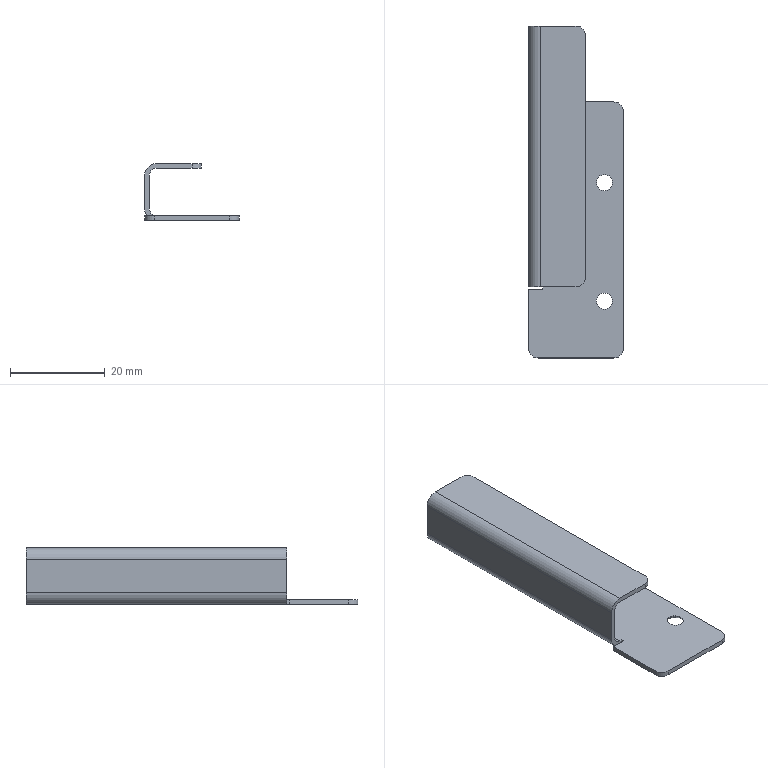Part | SolidWorks | features BaseBody 1 | 1 solid | 34 faces | box 20 x 70 x 12 mm | volume 2355 mm3 | plane 16 | cylinder 14 | cone 4 | commonest cylinder face diameters 4 x6 3.4 x4 3 x2 5 x2
STEP:
#1=CARTESIAN_POINT('',(-5.7,37.,1.));
#2=VERTEX_POINT('',#1);
#3=CARTESIAN_POINT('',(-2.3,37.,1.));
#4=VERTEX_POINT('',#3);
#5=CARTESIAN_POINT('',(-4.,37.,1.));
#6=DIRECTION('',(0.,0.,1.));
#7=DIRECTION('',(-1.,0.,0.));
#8=AXIS2_PLACEMENT_3D('',#5,#6,#7);
#9=CIRCLE('',#8,1.7);
#10=EDGE_CURVE('',#2,#4,#9,.T.);
#11=ORIENTED_EDGE('',*,*,#10,.T.);
#12=CARTESIAN_POINT('',(-2.3,37.,0.8));
#13=VERTEX_POINT('',#12);
#14=CARTESIAN_POINT('',(-2.3,37.,0.));
#15=DIRECTION('',(0.,0.,-1.));
#16=VECTOR('',#15,1000.);
#17=LINE('',#14,#16);
#18=EDGE_CURVE('',#4,#13,#17,.T.);
#19=ORIENTED_EDGE('',*,*,#18,.T.);
#20=CARTESIAN_POINT('',(-5.7,37.,0.8));
#21=VERTEX_POINT('',#20);
#22=CARTESIAN_POINT('',(-4.,37.,0.8));
#23=DIRECTION('',(0.,0.,1.));
#24=DIRECTION('',(-1.,0.,0.));
#25=AXIS2_PLACEMENT_3D('',#22,#23,#24);
#26=CIRCLE('',#25,1.7);
#27=EDGE_CURVE('',#21,#13,#26,.T.);
#28=ORIENTED_EDGE('',*,*,#27,.F.);
#29=CARTESIAN_POINT('',(-5.7,37.,0.));
#30=DIRECTION('',(0.,0.,-1.));
#31=VECTOR('',#30,1000.);
#32=LINE('',#29,#31);
#33=EDGE_CURVE('',#2,#21,#32,.T.);
#34=ORIENTED_EDGE('',*,*,#33,.F.);
#35=EDGE_LOOP('',(#11,#19,#28,#34));
#36=FACE_OUTER_BOUND('',#35,.T.);
#37=CARTESIAN_POINT('',(-4.,37.,0.));
#38=DIRECTION('',(0.,0.,-1.));
#39=DIRECTION('',(-1.,0.,0.));
#40=AXIS2_PLACEMENT_3D('',#37,#38,#39);
#41=CYLINDRICAL_SURFACE('',#40,1.7);
#42=ADVANCED_FACE('',(#36),#41,.F.);
#43=CARTESIAN_POINT('',(-5.7,12.,1.));
#44=VERTEX_POINT('',#43);
#45=CARTESIAN_POINT('',(-2.3,12.,1.));
#46=VERTEX_POINT('',#45);
#47=CARTESIAN_POINT('',(-4.,12.,1.));
#48=DIRECTION('',(0.,0.,1.));
#49=DIRECTION('',(-1.,0.,0.));
#50=AXIS2_PLACEMENT_3D('',#47,#48,#49);
#51=CIRCLE('',#50,1.7);
#52=EDGE_CURVE('',#44,#46,#51,.T.);
#53=ORIENTED_EDGE('',*,*,#52,.T.);
#54=CARTESIAN_POINT('',(-2.3,12.,0.8));
#55=VERTEX_POINT('',#54);
#56=CARTESIAN_POINT('',(-2.3,12.,0.));
#57=DIRECTION('',(0.,0.,-1.));
#58=VECTOR('',#57,1000.);
#59=LINE('',#56,#58);
#60=EDGE_CURVE('',#46,#55,#59,.T.);
#61=ORIENTED_EDGE('',*,*,#60,.T.);
#62=CARTESIAN_POINT('',(-5.7,12.,0.8));
#63=VERTEX_POINT('',#62);
#64=CARTESIAN_POINT('',(-4.,12.,0.8));
#65=DIRECTION('',(0.,0.,1.));
#66=DIRECTION('',(-1.,0.,0.));
#67=AXIS2_PLACEMENT_3D('',#64,#65,#66);
#68=CIRCLE('',#67,1.7);
#69=EDGE_CURVE('',#63,#55,#68,.T.);
#70=ORIENTED_EDGE('',*,*,#69,.F.);
#71=CARTESIAN_POINT('',(-5.7,12.,0.));
#72=DIRECTION('',(0.,0.,-1.));
#73=VECTOR('',#72,1000.);
#74=LINE('',#71,#73);
#75=EDGE_CURVE('',#44,#63,#74,.T.);
#76=ORIENTED_EDGE('',*,*,#75,.F.);
#77=EDGE_LOOP('',(#53,#61,#70,#76));
#78=FACE_OUTER_BOUND('',#77,.T.);
#79=CARTESIAN_POINT('',(-4.,12.,0.));
#80=DIRECTION('',(0.,0.,-1.));
#81=DIRECTION('',(-1.,0.,0.));
#82=AXIS2_PLACEMENT_3D('',#79,#80,#81);
#83=CYLINDRICAL_SURFACE('',#82,1.7);
#84=ADVANCED_FACE('',(#78),#83,.F.);
#85=ORIENTED_EDGE('',*,*,#27,.T.);
#86=CARTESIAN_POINT('',(-1.5,37.,0.));
#87=VERTEX_POINT('',#86);
#88=CARTESIAN_POINT('',(-1.5,37.,0.));
#89=DIRECTION('',(0.7071,0.,-0.7071));
#90=VECTOR('',#89,1000.);
#91=LINE('',#88,#90);
#92=EDGE_CURVE('',#13,#87,#91,.T.);
#93=ORIENTED_EDGE('',*,*,#92,.T.);
#94=CARTESIAN_POINT('',(-6.5,37.,0.));
#95=VERTEX_POINT('',#94);
#96=CARTESIAN_POINT('',(-4.,37.,0.));
#97=DIRECTION('',(0.,0.,1.));
#98=DIRECTION('',(-1.,0.,0.));
#99=AXIS2_PLACEMENT_3D('',#96,#97,#98);
#100=CIRCLE('',#99,2.5);
#101=EDGE_CURVE('',#95,#87,#100,.T.);
#102=ORIENTED_EDGE('',*,*,#101,.F.);
#103=CARTESIAN_POINT('',(-6.5,37.,0.));
#104=DIRECTION('',(-0.7071,0.,-0.7071));
#105=VECTOR('',#104,1000.);
#106=LINE('',#103,#105);
#107=EDGE_CURVE('',#21,#95,#106,.T.);
#108=ORIENTED_EDGE('',*,*,#107,.F.);
#109=EDGE_LOOP('',(#85,#93,#102,#108));
#110=FACE_OUTER_BOUND('',#109,.T.);
#111=CARTESIAN_POINT('',(-4.,37.,0.));
#112=DIRECTION('',(0.,0.,-1.));
#113=DIRECTION('',(-1.,0.,0.));
#114=AXIS2_PLACEMENT_3D('',#111,#112,#113);
#115=CONICAL_SURFACE('',#114,2.5,0.7854);
#116=ADVANCED_FACE('',(#110),#115,.F.);
#117=ORIENTED_EDGE('',*,*,#69,.T.);
#118=CARTESIAN_POINT('',(-1.5,12.,0.));
#119=VERTEX_POINT('',#118);
#120=CARTESIAN_POINT('',(-1.5,12.,0.));
#121=DIRECTION('',(0.7071,0.,-0.7071));
#122=VECTOR('',#121,1000.);
#123=LINE('',#120,#122);
#124=EDGE_CURVE('',#55,#119,#123,.T.);
#125=ORIENTED_EDGE('',*,*,#124,.T.);
#126=CARTESIAN_POINT('',(-6.5,12.,0.));
#127=VERTEX_POINT('',#126);
#128=CARTESIAN_POINT('',(-4.,12.,0.));
#129=DIRECTION('',(0.,0.,1.));
#130=DIRECTION('',(-1.,0.,0.));
#131=AXIS2_PLACEMENT_3D('',#128,#129,#130);
#132=CIRCLE('',#131,2.5);
#133=EDGE_CURVE('',#127,#119,#132,.T.);
#134=ORIENTED_EDGE('',*,*,#133,.F.);
#135=CARTESIAN_POINT('',(-6.5,12.,0.));
#136=DIRECTION('',(-0.7071,0.,-0.7071));
#137=VECTOR('',#136,1000.);
#138=LINE('',#135,#137);
#139=EDGE_CURVE('',#63,#127,#138,.T.);
#140=ORIENTED_EDGE('',*,*,#139,.F.);
#141=EDGE_LOOP('',(#117,#125,#134,#140));
#142=FACE_OUTER_BOUND('',#141,.T.);
#143=CARTESIAN_POINT('',(-4.,12.,0.));
#144=DIRECTION('',(0.,0.,-1.));
#145=DIRECTION('',(-1.,0.,0.));
#146=AXIS2_PLACEMENT_3D('',#143,#144,#145);
#147=CONICAL_SURFACE('',#146,2.5,0.7854);
#148=ADVANCED_FACE('',(#142),#147,.F.);
#149=ORIENTED_EDGE('',*,*,#10,.F.);
#150=CARTESIAN_POINT('',(-4.,37.,1.));
#151=DIRECTION('',(0.,0.,1.));
#152=DIRECTION('',(-1.,0.,0.));
#153=AXIS2_PLACEMENT_3D('',#150,#151,#152);
#154=CIRCLE('',#153,1.7);
#155=EDGE_CURVE('',#4,#2,#154,.T.);
#156=ORIENTED_EDGE('',*,*,#155,.F.);
#157=EDGE_LOOP('',(#149,#156));
#158=FACE_BOUND('',#157,.T.);
#159=ORIENTED_EDGE('',*,*,#52,.F.);
#160=CARTESIAN_POINT('',(-4.,12.,1.));
#161=DIRECTION('',(0.,0.,1.));
#162=DIRECTION('',(-1.,0.,0.));
#163=AXIS2_PLACEMENT_3D('',#160,#161,#162);
#164=CIRCLE('',#163,1.7);
#165=EDGE_CURVE('',#46,#44,#164,.T.);
#166=ORIENTED_EDGE('',*,*,#165,.F.);
#167=EDGE_LOOP('',(#159,#166));
#168=FACE_BOUND('',#167,.T.);
#169=CARTESIAN_POINT('',(0.,52.,1.));
#170=VERTEX_POINT('',#169);
#171=CARTESIAN_POINT('',(0.,2.,1.));
#172=VERTEX_POINT('',#171);
#173=CARTESIAN_POINT('',(0.,70.,1.));
#174=DIRECTION('',(0.,-1.,0.));
#175=VECTOR('',#174,1000.);
#176=LINE('',#173,#175);
#177=EDGE_CURVE('',#170,#172,#176,.T.);
#178=ORIENTED_EDGE('',*,*,#177,.F.);
#179=CARTESIAN_POINT('',(-2.,54.,1.));
#180=VERTEX_POINT('',#179);
#181=CARTESIAN_POINT('',(-2.,52.,1.));
#182=DIRECTION('',(0.,0.,-1.));
#183=DIRECTION('',(-1.,0.,0.));
#184=AXIS2_PLACEMENT_3D('',#181,#182,#183);
#185=CIRCLE('',#184,2.);
#186=EDGE_CURVE('',#180,#170,#185,.T.);
#187=ORIENTED_EDGE('',*,*,#186,.F.);
#188=CARTESIAN_POINT('',(-8.,54.,1.));
#189=VERTEX_POINT('',#188);
#190=CARTESIAN_POINT('',(0.,54.,1.));
#191=DIRECTION('',(1.,0.,0.));
#192=VECTOR('',#191,1000.);
#193=LINE('',#190,#192);
#194=EDGE_CURVE('',#189,#180,#193,.T.);
#195=ORIENTED_EDGE('',*,*,#194,.F.);
#196=CARTESIAN_POINT('',(-8.,68.,1.));
#197=VERTEX_POINT('',#196);
#198=CARTESIAN_POINT('',(-8.,70.,1.));
#199=DIRECTION('',(0.,-1.,0.));
#200=VECTOR('',#199,1000.);
#201=LINE('',#198,#200);
#202=EDGE_CURVE('',#197,#189,#201,.T.);
#203=ORIENTED_EDGE('',*,*,#202,.F.);
#204=CARTESIAN_POINT('',(-10.,70.,1.));
#205=VERTEX_POINT('',#204);
#206=CARTESIAN_POINT('',(-10.,68.,1.));
#207=DIRECTION('',(0.,0.,-1.));
#208=DIRECTION('',(-1.,0.,0.));
#209=AXIS2_PLACEMENT_3D('',#206,#207,#208);
#210=CIRCLE('',#209,2.);
#211=EDGE_CURVE('',#205,#197,#210,.T.);
#212=ORIENTED_EDGE('',*,*,#211,.F.);
#213=CARTESIAN_POINT('',(-17.5,70.,1.));
#214=VERTEX_POINT('',#213);
#215=CARTESIAN_POINT('',(0.,70.,1.));
#216=DIRECTION('',(1.,0.,0.));
#217=VECTOR('',#216,1000.);
#218=LINE('',#215,#217);
#219=EDGE_CURVE('',#214,#205,#218,.T.);
#220=ORIENTED_EDGE('',*,*,#219,.F.);
#221=CARTESIAN_POINT('',(-17.5,15.,1.));
#222=VERTEX_POINT('',#221);
#223=CARTESIAN_POINT('',(-17.5,70.,1.));
#224=DIRECTION('',(0.,1.,0.));
#225=VECTOR('',#224,1000.);
#226=LINE('',#223,#225);
#227=EDGE_CURVE('',#222,#214,#226,.T.);
#228=ORIENTED_EDGE('',*,*,#227,.F.);
#229=CARTESIAN_POINT('',(-17.,15.,1.));
#230=VERTEX_POINT('',#229);
#231=CARTESIAN_POINT('',(-8.,15.,1.));
#232=DIRECTION('',(1.,0.,0.));
#233=VECTOR('',#232,1000.);
#234=LINE('',#231,#233);
#235=EDGE_CURVE('',#222,#230,#234,.T.);
#236=ORIENTED_EDGE('',*,*,#235,.T.);
#237=CARTESIAN_POINT('',(-17.,14.5,1.));
#238=VERTEX_POINT('',#237);
#239=CARTESIAN_POINT('',(-17.,70.,1.));
#240=DIRECTION('',(0.,1.,0.));
#241=VECTOR('',#240,1000.);
#242=LINE('',#239,#241);
#243=EDGE_CURVE('',#238,#230,#242,.T.);
#244=ORIENTED_EDGE('',*,*,#243,.F.);
#245=CARTESIAN_POINT('',(-20.,14.5,1.));
#246=VERTEX_POINT('',#245);
#247=CARTESIAN_POINT('',(0.,14.5,1.));
#248=DIRECTION('',(1.,0.,0.));
#249=VECTOR('',#248,1000.);
#250=LINE('',#247,#249);
#251=EDGE_CURVE('',#246,#238,#250,.T.);
#252=ORIENTED_EDGE('',*,*,#251,.F.);
#253=CARTESIAN_POINT('',(-20.,2.,1.));
#254=VERTEX_POINT('',#253);
#255=CARTESIAN_POINT('',(-20.,70.,1.));
#256=DIRECTION('',(0.,1.,0.));
#257=VECTOR('',#256,1000.);
#258=LINE('',#255,#257);
#259=EDGE_CURVE('',#254,#246,#258,.T.);
#260=ORIENTED_EDGE('',*,*,#259,.F.);
#261=CARTESIAN_POINT('',(-18.,0.,1.));
#262=VERTEX_POINT('',#261);
#263=CARTESIAN_POINT('',(-18.,2.,1.));
#264=DIRECTION('',(0.,0.,-1.));
#265=DIRECTION('',(-1.,0.,0.));
#266=AXIS2_PLACEMENT_3D('',#263,#264,#265);
#267=CIRCLE('',#266,2.);
#268=EDGE_CURVE('',#262,#254,#267,.T.);
#269=ORIENTED_EDGE('',*,*,#268,.F.);
#270=CARTESIAN_POINT('',(-2.,0.,1.));
#271=VERTEX_POINT('',#270);
#272=CARTESIAN_POINT('',(0.,0.,1.));
#273=DIRECTION('',(-1.,0.,0.));
#274=VECTOR('',#273,1000.);
#275=LINE('',#272,#274);
#276=EDGE_CURVE('',#271,#262,#275,.T.);
#277=ORIENTED_EDGE('',*,*,#276,.F.);
#278=CARTESIAN_POINT('',(-2.,2.,1.));
#279=DIRECTION('',(0.,0.,-1.));
#280=DIRECTION('',(1.,0.,0.));
#281=AXIS2_PLACEMENT_3D('',#278,#279,#280);
#282=CIRCLE('',#281,2.);
#283=EDGE_CURVE('',#172,#271,#282,.T.);
#284=ORIENTED_EDGE('',*,*,#283,.F.);
#285=EDGE_LOOP('',(#178,#187,#195,#203,#212,#220,#228,#236,#244,#252,#260,#269,#277,#284));
#286=FACE_OUTER_BOUND('',#285,.T.);
#287=CARTESIAN_POINT('',(0.,70.,1.));
#288=DIRECTION('',(0.,0.,-1.));
#289=DIRECTION('',(-1.,0.,0.));
#290=AXIS2_PLACEMENT_3D('',#287,#288,#289);
#291=PLANE('',#290);
#292=ADVANCED_FACE('',(#158,#168,#286),#291,.F.);
#293=ORIENTED_EDGE('',*,*,#18,.F.);
#294=ORIENTED_EDGE('',*,*,#155,.T.);
#295=ORIENTED_EDGE('',*,*,#33,.T.);
#296=CARTESIAN_POINT('',(-4.,37.,0.8));
#297=DIRECTION('',(0.,0.,1.));
#298=DIRECTION('',(-1.,0.,0.));
#299=AXIS2_PLACEMENT_3D('',#296,#297,#298);
#300=CIRCLE('',#299,1.7);
#301=EDGE_CURVE('',#13,#21,#300,.T.);
#302=ORIENTED_EDGE('',*,*,#301,.F.);
#303=EDGE_LOOP('',(#293,#294,#295,#302));
#304=FACE_OUTER_BOUND('',#303,.T.);
#305=CARTESIAN_POINT('',(-4.,37.,0.));
#306=DIRECTION('',(0.,0.,-1.));
#307=DIRECTION('',(-1.,0.,0.));
#308=AXIS2_PLACEMENT_3D('',#305,#306,#307);
#309=CYLINDRICAL_SURFACE('',#308,1.7);
#310=ADVANCED_FACE('',(#304),#309,.F.);
#311=ORIENTED_EDGE('',*,*,#60,.F.);
#312=ORIENTED_EDGE('',*,*,#165,.T.);
#313=ORIENTED_EDGE('',*,*,#75,.T.);
#314=CARTESIAN_POINT('',(-4.,12.,0.8));
#315=DIRECTION('',(0.,0.,1.));
#316=DIRECTION('',(-1.,0.,0.));
#317=AXIS2_PLACEMENT_3D('',#314,#315,#316);
#318=CIRCLE('',#317,1.7);
#319=EDGE_CURVE('',#55,#63,#318,.T.);
#320=ORIENTED_EDGE('',*,*,#319,.F.);
#321=EDGE_LOOP('',(#311,#312,#313,#320));
#322=FACE_OUTER_BOUND('',#321,.T.);
#323=CARTESIAN_POINT('',(-4.,12.,0.));
#324=DIRECTION('',(0.,0.,-1.));
#325=DIRECTION('',(-1.,0.,0.));
#326=AXIS2_PLACEMENT_3D('',#323,#324,#325);
#327=CYLINDRICAL_SURFACE('',#326,1.7);
#328=ADVANCED_FACE('',(#322),#327,.F.);
#329=ORIENTED_EDGE('',*,*,#283,.T.);
#330=CARTESIAN_POINT('',(-2.,0.,0.));
#331=VERTEX_POINT('',#330);
#332=CARTESIAN_POINT('',(-2.,0.,0.));
#333=DIRECTION('',(0.,0.,-1.));
#334=VECTOR('',#333,1000.);
#335=LINE('',#332,#334);
#336=EDGE_CURVE('',#271,#331,#335,.T.);
#337=ORIENTED_EDGE('',*,*,#336,.T.);
#338=CARTESIAN_POINT('',(0.,2.,0.));
#339=VERTEX_POINT('',#338);
#340=CARTESIAN_POINT('',(-2.,2.,0.));
#341=DIRECTION('',(0.,0.,1.));
#342=DIRECTION('',(1.,0.,0.));
#343=AXIS2_PLACEMENT_3D('',#340,#341,#342);
#344=CIRCLE('',#343,2.);
#345=EDGE_CURVE('',#331,#339,#344,.T.);
#346=ORIENTED_EDGE('',*,*,#345,.T.);
#347=CARTESIAN_POINT('',(0.,2.,0.));
#348=DIRECTION('',(0.,0.,1.));
#349=VECTOR('',#348,1000.);
#350=LINE('',#347,#349);
#351=EDGE_CURVE('',#339,#172,#350,.T.);
#352=ORIENTED_EDGE('',*,*,#351,.T.);
#353=EDGE_LOOP('',(#329,#337,#346,#352));
#354=FACE_OUTER_BOUND('',#353,.T.);
#355=CARTESIAN_POINT('',(-2.,2.,0.));
#356=DIRECTION('',(0.,0.,1.));
#357=DIRECTION('',(1.,0.,0.));
#358=AXIS2_PLACEMENT_3D('',#355,#356,#357);
#359=CYLINDRICAL_SURFACE('',#358,2.);
#360=ADVANCED_FACE('',(#354),#359,.T.);
#361=ORIENTED_EDGE('',*,*,#177,.T.);
#362=ORIENTED_EDGE('',*,*,#351,.F.);
#363=CARTESIAN_POINT('',(0.,52.,0.));
#364=VERTEX_POINT('',#363);
#365=CARTESIAN_POINT('',(0.,70.,0.));
#366=DIRECTION('',(0.,-1.,0.));
#367=VECTOR('',#366,1000.);
#368=LINE('',#365,#367);
#369=EDGE_CURVE('',#364,#339,#368,.T.);
#370=ORIENTED_EDGE('',*,*,#369,.F.);
#371=CARTESIAN_POINT('',(0.,52.,0.));
#372=DIRECTION('',(0.,0.,-1.));
#373=VECTOR('',#372,1000.);
#374=LINE('',#371,#373);
#375=EDGE_CURVE('',#170,#364,#374,.T.);
#376=ORIENTED_EDGE('',*,*,#375,.F.);
#377=EDGE_LOOP('',(#361,#362,#370,#376));
#378=FACE_OUTER_BOUND('',#377,.T.);
#379=CARTESIAN_POINT('',(0.,70.,0.));
#380=DIRECTION('',(-1.,0.,0.));
#381=DIRECTION('',(0.,0.,1.));
#382=AXIS2_PLACEMENT_3D('',#379,#380,#381);
#383=PLANE('',#382);
#384=ADVANCED_FACE('',(#378),#383,.F.);
#385=ORIENTED_EDGE('',*,*,#186,.T.);
#386=ORIENTED_EDGE('',*,*,#375,.T.);
#387=CARTESIAN_POINT('',(-2.,54.,0.));
#388=VERTEX_POINT('',#387);
#389=CARTESIAN_POINT('',(-2.,52.,0.));
#390=DIRECTION('',(0.,0.,1.));
#391=DIRECTION('',(-1.,0.,0.));
#392=AXIS2_PLACEMENT_3D('',#389,#390,#391);
#393=CIRCLE('',#392,2.);
#394=EDGE_CURVE('',#364,#388,#393,.T.);
#395=ORIENTED_EDGE('',*,*,#394,.T.);
#396=CARTESIAN_POINT('',(-2.,54.,2.));
#397=DIRECTION('',(0.,0.,1.));
#398=VECTOR('',#397,1000.);
#399=LINE('',#396,#398);
#400=EDGE_CURVE('',#388,#180,#399,.T.);
#401=ORIENTED_EDGE('',*,*,#400,.T.);
#402=EDGE_LOOP('',(#385,#386,#395,#401));
#403=FACE_OUTER_BOUND('',#402,.T.);
#404=CARTESIAN_POINT('',(-2.,52.,2.));
#405=DIRECTION('',(0.,0.,-1.));
#406=DIRECTION('',(-1.,0.,0.));
#407=AXIS2_PLACEMENT_3D('',#404,#405,#406);
#408=CYLINDRICAL_SURFACE('',#407,2.);
#409=ADVANCED_FACE('',(#403),#408,.T.);
#410=ORIENTED_EDGE('',*,*,#194,.T.);
#411=ORIENTED_EDGE('',*,*,#400,.F.);
#412=CARTESIAN_POINT('',(-8.,54.,0.));
#413=VERTEX_POINT('',#412);
#414=CARTESIAN_POINT('',(0.,54.,0.));
#415=DIRECTION('',(1.,0.,0.));
#416=VECTOR('',#415,1000.);
#417=LINE('',#414,#416);
#418=EDGE_CURVE('',#413,#388,#417,.T.);
#419=ORIENTED_EDGE('',*,*,#418,.F.);
#420=CARTESIAN_POINT('',(-8.,54.,2.));
#421=DIRECTION('',(0.,0.,-1.));
#422=VECTOR('',#421,1000.);
#423=LINE('',#420,#422);
#424=EDGE_CURVE('',#189,#413,#423,.T.);
#425=ORIENTED_EDGE('',*,*,#424,.F.);
#426=EDGE_LOOP('',(#410,#411,#419,#425));
#427=FACE_OUTER_BOUND('',#426,.T.);
#428=CARTESIAN_POINT('',(0.,54.,2.));
#429=DIRECTION('',(0.,-1.,0.));
#430=DIRECTION('',(0.,0.,-1.));
#431=AXIS2_PLACEMENT_3D('',#428,#429,#430);
#432=PLANE('',#431);
#433=ADVANCED_FACE('',(#427),#432,.F.);
#434=CARTESIAN_POINT('',(-8.,68.,0.));
#435=VERTEX_POINT('',#434);
#436=CARTESIAN_POINT('',(-8.,70.,0.));
#437=DIRECTION('',(0.,-1.,0.));
#438=VECTOR('',#437,1000.);
#439=LINE('',#436,#438);
#440=EDGE_CURVE('',#435,#413,#439,.T.);
#441=ORIENTED_EDGE('',*,*,#440,.F.);
#442=CARTESIAN_POINT('',(-8.,68.,2.));
#443=DIRECTION('',(0.,0.,-1.));
#444=VECTOR('',#443,1000.);
#445=LINE('',#442,#444);
#446=EDGE_CURVE('',#197,#435,#445,.T.);
#447=ORIENTED_EDGE('',*,*,#446,.F.);
#448=ORIENTED_EDGE('',*,*,#202,.T.);
#449=ORIENTED_EDGE('',*,*,#424,.T.);
#450=EDGE_LOOP('',(#441,#447,#448,#449));
#451=FACE_OUTER_BOUND('',#450,.T.);
#452=CARTESIAN_POINT('',(-8.,70.,2.));
#453=DIRECTION('',(-1.,0.,0.));
#454=DIRECTION('',(0.,0.,1.));
#455=AXIS2_PLACEMENT_3D('',#452,#453,#454);
#456=PLANE('',#455);
#457=ADVANCED_FACE('',(#451),#456,.F.);
#458=ORIENTED_EDGE('',*,*,#211,.T.);
#459=ORIENTED_EDGE('',*,*,#446,.T.);
#460=CARTESIAN_POINT('',(-10.,70.,0.));
#461=VERTEX_POINT('',#460);
#462=CARTESIAN_POINT('',(-10.,68.,0.));
#463=DIRECTION('',(0.,0.,1.));
#464=DIRECTION('',(-1.,0.,0.));
#465=AXIS2_PLACEMENT_3D('',#462,#463,#464);
#466=CIRCLE('',#465,2.);
#467=EDGE_CURVE('',#435,#461,#466,.T.);
#468=ORIENTED_EDGE('',*,*,#467,.T.);
#469=CARTESIAN_POINT('',(-10.,70.,0.));
#470=DIRECTION('',(0.,0.,1.));
#471=VECTOR('',#470,1000.);
#472=LINE('',#469,#471);
#473=EDGE_CURVE('',#461,#205,#472,.T.);
#474=ORIENTED_EDGE('',*,*,#473,.T.);
#475=EDGE_LOOP('',(#458,#459,#468,#474));
#476=FACE_OUTER_BOUND('',#475,.T.);
#477=CARTESIAN_POINT('',(-10.,68.,0.));
#478=DIRECTION('',(0.,0.,-1.));
#479=DIRECTION('',(-1.,0.,0.));
#480=AXIS2_PLACEMENT_3D('',#477,#478,#479);
#481=CYLINDRICAL_SURFACE('',#480,2.);
#482=ADVANCED_FACE('',(#476),#481,.T.);
#483=CARTESIAN_POINT('',(-17.5,70.,11.));
#484=VERTEX_POINT('',#483);
#485=CARTESIAN_POINT('',(-10.,70.,11.));
#486=VERTEX_POINT('',#485);
#487=CARTESIAN_POINT('',(0.,70.,11.));
#488=DIRECTION('',(1.,0.,0.));
#489=VECTOR('',#488,1000.);
#490=LINE('',#487,#489);
#491=EDGE_CURVE('',#484,#486,#490,.T.);
#492=ORIENTED_EDGE('',*,*,#491,.F.);
#493=CARTESIAN_POINT('',(-19.,70.,9.5));
#494=VERTEX_POINT('',#493);
#495=CARTESIAN_POINT('',(-17.5,70.,9.5));
#496=DIRECTION('',(0.,1.,0.));
#497=DIRECTION('',(0.,0.,1.));
#498=AXIS2_PLACEMENT_3D('',#495,#496,#497);
#499=CIRCLE('',#498,1.5);
#500=EDGE_CURVE('',#494,#484,#499,.T.);
#501=ORIENTED_EDGE('',*,*,#500,.F.);
#502=CARTESIAN_POINT('',(-19.,70.,2.5));
#503=VERTEX_POINT('',#502);
#504=CARTESIAN_POINT('',(-19.,70.,0.));
#505=DIRECTION('',(0.,0.,1.));
#506=VECTOR('',#505,1000.);
#507=LINE('',#504,#506);
#508=EDGE_CURVE('',#503,#494,#507,.T.);
#509=ORIENTED_EDGE('',*,*,#508,.F.);
#510=CARTESIAN_POINT('',(-17.5,70.,2.5));
#511=DIRECTION('',(0.,1.,0.));
#512=DIRECTION('',(0.,0.,1.));
#513=AXIS2_PLACEMENT_3D('',#510,#511,#512);
#514=CIRCLE('',#513,1.5);
#515=EDGE_CURVE('',#214,#503,#514,.T.);
#516=ORIENTED_EDGE('',*,*,#515,.F.);
#517=ORIENTED_EDGE('',*,*,#219,.T.);
#518=ORIENTED_EDGE('',*,*,#473,.F.);
#519=CARTESIAN_POINT('',(-17.5,70.,0.));
#520=VERTEX_POINT('',#519);
#521=CARTESIAN_POINT('',(0.,70.,0.));
#522=DIRECTION('',(1.,0.,0.));
#523=VECTOR('',#522,1000.);
#524=LINE('',#521,#523);
#525=EDGE_CURVE('',#520,#461,#524,.T.);
#526=ORIENTED_EDGE('',*,*,#525,.F.);
#527=CARTESIAN_POINT('',(-20.,70.,2.5));
#528=VERTEX_POINT('',#527);
#529=CARTESIAN_POINT('',(-17.5,70.,2.5));
#530=DIRECTION('',(0.,-1.,0.));
#531=DIRECTION('',(0.,0.,-1.));
#532=AXIS2_PLACEMENT_3D('',#529,#530,#531);
#533=CIRCLE('',#532,2.5);
#534=EDGE_CURVE('',#528,#520,#533,.T.);
#535=ORIENTED_EDGE('',*,*,#534,.F.);
#536=CARTESIAN_POINT('',(-20.,70.,9.5));
#537=VERTEX_POINT('',#536);
#538=CARTESIAN_POINT('',(-20.,70.,0.));
#539=DIRECTION('',(0.,0.,-1.));
#540=VECTOR('',#539,1000.);
#541=LINE('',#538,#540);
#542=EDGE_CURVE('',#537,#528,#541,.T.);
#543=ORIENTED_EDGE('',*,*,#542,.F.);
#544=CARTESIAN_POINT('',(-17.5,70.,12.));
#545=VERTEX_POINT('',#544);
#546=CARTESIAN_POINT('',(-17.5,70.,9.5));
#547=DIRECTION('',(0.,-1.,0.));
#548=DIRECTION('',(0.,0.,-1.));
#549=AXIS2_PLACEMENT_3D('',#546,#547,#548);
#550=CIRCLE('',#549,2.5);
#551=EDGE_CURVE('',#545,#537,#550,.T.);
#552=ORIENTED_EDGE('',*,*,#551,.F.);
#553=CARTESIAN_POINT('',(-10.,70.,12.));
#554=VERTEX_POINT('',#553);
#555=CARTESIAN_POINT('',(0.,70.,12.));
#556=DIRECTION('',(-1.,0.,0.));
#557=VECTOR('',#556,1000.);
#558=LINE('',#555,#557);
#559=EDGE_CURVE('',#554,#545,#558,.T.);
#560=ORIENTED_EDGE('',*,*,#559,.F.);
#561=CARTESIAN_POINT('',(-10.,70.,0.));
#562=DIRECTION('',(0.,0.,1.));
#563=VECTOR('',#562,1000.);
#564=LINE('',#561,#563);
#565=EDGE_CURVE('',#486,#554,#564,.T.);
#566=ORIENTED_EDGE('',*,*,#565,.F.);
#567=EDGE_LOOP('',(#492,#501,#509,#516,#517,#518,#526,#535,#543,#552,#560,#566));
#568=FACE_OUTER_BOUND('',#567,.T.);
#569=CARTESIAN_POINT('',(0.,70.,0.));
#570=DIRECTION('',(0.,-1.,0.));
#571=DIRECTION('',(0.,0.,-1.));
#572=AXIS2_PLACEMENT_3D('',#569,#570,#571);
#573=PLANE('',#572);
#574=ADVANCED_FACE('',(#568),#573,.F.);
#575=ORIENTED_EDGE('',*,*,#515,.T.);
#576=CARTESIAN_POINT('',(-19.,15.,2.5));
#577=VERTEX_POINT('',#576);
#578=CARTESIAN_POINT('',(-19.,70.,2.5));
#579=DIRECTION('',(0.,1.,0.));
#580=VECTOR('',#579,1000.);
#581=LINE('',#578,#580);
#582=EDGE_CURVE('',#577,#503,#581,.T.);
#583=ORIENTED_EDGE('',*,*,#582,.F.);
#584=CARTESIAN_POINT('',(-17.5,15.,2.5));
#585=DIRECTION('',(0.,1.,0.));
#586=DIRECTION('',(0.,0.,1.));
#587=AXIS2_PLACEMENT_3D('',#584,#585,#586);
#588=CIRCLE('',#587,1.5);
#589=EDGE_CURVE('',#222,#577,#588,.T.);
#590=ORIENTED_EDGE('',*,*,#589,.F.);
#591=ORIENTED_EDGE('',*,*,#227,.T.);
#592=EDGE_LOOP('',(#575,#583,#590,#591));
#593=FACE_OUTER_BOUND('',#592,.T.);
#594=CARTESIAN_POINT('',(-17.5,70.,2.5));
#595=DIRECTION('',(0.,1.,0.));
#596=DIRECTION('',(0.,0.,1.));
#597=AXIS2_PLACEMENT_3D('',#594,#595,#596);
#598=CYLINDRICAL_SURFACE('',#597,1.5);
#599=ADVANCED_FACE('',(#593),#598,.F.);
#600=CARTESIAN_POINT('',(-17.,14.5,0.));
#601=VERTEX_POINT('',#600);
#602=CARTESIAN_POINT('',(-17.,14.5,-10.));
#603=DIRECTION('',(0.,0.,-1.));
#604=VECTOR('',#603,1000.);
#605=LINE('',#602,#604);
#606=EDGE_CURVE('',#238,#601,#605,.T.);
#607=ORIENTED_EDGE('',*,*,#606,.F.);
#608=ORIENTED_EDGE('',*,*,#243,.T.);
#609=CARTESIAN_POINT('',(-17.,15.,0.));
#610=VERTEX_POINT('',#609);
#611=CARTESIAN_POINT('',(-17.,15.,-10.));
#612=DIRECTION('',(0.,0.,1.));
#613=VECTOR('',#612,1000.);
#614=LINE('',#611,#613);
#615=EDGE_CURVE('',#610,#230,#614,.T.);
#616=ORIENTED_EDGE('',*,*,#615,.F.);
#617=CARTESIAN_POINT('',(-17.,15.,0.));
#618=DIRECTION('',(0.,1.,0.));
#619=VECTOR('',#618,1000.);
#620=LINE('',#617,#619);
#621=EDGE_CURVE('',#601,#610,#620,.T.);
#622=ORIENTED_EDGE('',*,*,#621,.F.);
#623=EDGE_LOOP('',(#607,#608,#616,#622));
#624=FACE_OUTER_BOUND('',#623,.T.);
#625=CARTESIAN_POINT('',(-17.,15.,-10.));
#626=DIRECTION('',(1.,0.,0.));
#627=DIRECTION('',(0.,0.,-1.));
#628=AXIS2_PLACEMENT_3D('',#625,#626,#627);
#629=PLANE('',#628);
#630=ADVANCED_FACE('',(#624),#629,.F.);
#631=CARTESIAN_POINT('',(-20.,14.5,0.));
#632=VERTEX_POINT('',#631);
#633=CARTESIAN_POINT('',(-20.,14.5,-10.));
#634=DIRECTION('',(0.,0.,-1.));
#635=VECTOR('',#634,1000.);
#636=LINE('',#633,#635);
#637=EDGE_CURVE('',#246,#632,#636,.T.);
#638=ORIENTED_EDGE('',*,*,#637,.F.);
#639=ORIENTED_EDGE('',*,*,#251,.T.);
#640=ORIENTED_EDGE('',*,*,#606,.T.);
#641=CARTESIAN_POINT('',(-17.,14.5,0.));
#642=DIRECTION('',(1.,0.,0.));
#643=VECTOR('',#642,1000.);
#644=LINE('',#641,#643);
#645=EDGE_CURVE('',#632,#601,#644,.T.);
#646=ORIENTED_EDGE('',*,*,#645,.F.);
#647=EDGE_LOOP('',(#638,#639,#640,#646));
#648=FACE_OUTER_BOUND('',#647,.T.);
#649=CARTESIAN_POINT('',(-17.,14.5,-10.));
#650=DIRECTION('',(0.,-1.,0.));
#651=DIRECTION('',(1.,0.,0.));
#652=AXIS2_PLACEMENT_3D('',#649,#650,#651);
#653=PLANE('',#652);
#654=ADVANCED_FACE('',(#648),#653,.F.);
#655=CARTESIAN_POINT('',(-20.,2.,0.));
#656=VERTEX_POINT('',#655);
#657=CARTESIAN_POINT('',(-20.,70.,0.));
#658=DIRECTION('',(0.,1.,0.));
#659=VECTOR('',#658,1000.);
#660=LINE('',#657,#659);
#661=EDGE_CURVE('',#656,#632,#660,.T.);
#662=ORIENTED_EDGE('',*,*,#661,.F.);
#663=CARTESIAN_POINT('',(-20.,2.,0.));
#664=DIRECTION('',(0.,0.,-1.));
#665=VECTOR('',#664,1000.);
#666=LINE('',#663,#665);
#667=EDGE_CURVE('',#254,#656,#666,.T.);
#668=ORIENTED_EDGE('',*,*,#667,.F.);
#669=ORIENTED_EDGE('',*,*,#259,.T.);
#670=ORIENTED_EDGE('',*,*,#637,.T.);
#671=EDGE_LOOP('',(#662,#668,#669,#670));
#672=FACE_OUTER_BOUND('',#671,.T.);
#673=CARTESIAN_POINT('',(-20.,70.,0.));
#674=DIRECTION('',(1.,0.,0.));
#675=DIRECTION('',(0.,0.,-1.));
#676=AXIS2_PLACEMENT_3D('',#673,#674,#675);
#677=PLANE('',#676);
#678=ADVANCED_FACE('',(#672),#677,.F.);
#679=CARTESIAN_POINT('',(-18.,0.,0.));
#680=VERTEX_POINT('',#679);
#681=CARTESIAN_POINT('',(-18.,2.,0.));
#682=DIRECTION('',(0.,0.,1.));
#683=DIRECTION('',(-1.,0.,0.));
#684=AXIS2_PLACEMENT_3D('',#681,#682,#683);
#685=CIRCLE('',#684,2.);
#686=EDGE_CURVE('',#656,#680,#685,.T.);
#687=ORIENTED_EDGE('',*,*,#686,.T.);
#688=CARTESIAN_POINT('',(-18.,0.,0.));
#689=DIRECTION('',(0.,0.,1.));
#690=VECTOR('',#689,1000.);
#691=LINE('',#688,#690);
#692=EDGE_CURVE('',#680,#262,#691,.T.);
#693=ORIENTED_EDGE('',*,*,#692,.T.);
#694=ORIENTED_EDGE('',*,*,#268,.T.);
#695=ORIENTED_EDGE('',*,*,#667,.T.);
#696=EDGE_LOOP('',(#687,#693,#694,#695));
#697=FACE_OUTER_BOUND('',#696,.T.);
#698=CARTESIAN_POINT('',(-18.,2.,0.));
#699=DIRECTION('',(0.,0.,-1.));
#700=DIRECTION('',(-1.,0.,0.));
#701=AXIS2_PLACEMENT_3D('',#698,#699,#700);
#702=CYLINDRICAL_SURFACE('',#701,2.);
#703=ADVANCED_FACE('',(#697),#702,.T.);
#704=ORIENTED_EDGE('',*,*,#276,.T.);
#705=ORIENTED_EDGE('',*,*,#692,.F.);
#706=CARTESIAN_POINT('',(0.,0.,0.));
#707=DIRECTION('',(1.,0.,0.));
#708=VECTOR('',#707,1000.);
#709=LINE('',#706,#708);
#710=EDGE_CURVE('',#680,#331,#709,.T.);
#711=ORIENTED_EDGE('',*,*,#710,.T.);
#712=ORIENTED_EDGE('',*,*,#336,.F.);
#713=EDGE_LOOP('',(#704,#705,#711,#712));
#714=FACE_OUTER_BOUND('',#713,.T.);
#715=CARTESIAN_POINT('',(0.,0.,0.));
#716=DIRECTION('',(0.,-1.,0.));
#717=DIRECTION('',(0.,0.,-1.));
#718=AXIS2_PLACEMENT_3D('',#715,#716,#717);
#719=PLANE('',#718);
#720=ADVANCED_FACE('',(#714),#719,.T.);
#721=ORIENTED_EDGE('',*,*,#92,.F.);
#722=ORIENTED_EDGE('',*,*,#301,.T.);
#723=ORIENTED_EDGE('',*,*,#107,.T.);
#724=CARTESIAN_POINT('',(-4.,37.,0.));
#725=DIRECTION('',(0.,0.,1.));
#726=DIRECTION('',(-1.,0.,0.));
#727=AXIS2_PLACEMENT_3D('',#724,#725,#726);
#728=CIRCLE('',#727,2.5);
#729=EDGE_CURVE('',#87,#95,#728,.T.);
#730=ORIENTED_EDGE('',*,*,#729,.F.);
#731=EDGE_LOOP('',(#721,#722,#723,#730));
#732=FACE_OUTER_BOUND('',#731,.T.);
#733=CARTESIAN_POINT('',(-4.,37.,0.));
#734=DIRECTION('',(0.,0.,-1.));
#735=DIRECTION('',(-1.,0.,0.));
#736=AXIS2_PLACEMENT_3D('',#733,#734,#735);
#737=CONICAL_SURFACE('',#736,2.5,0.7854);
#738=ADVANCED_FACE('',(#732),#737,.F.);
#739=ORIENTED_EDGE('',*,*,#124,.F.);
#740=ORIENTED_EDGE('',*,*,#319,.T.);
#741=ORIENTED_EDGE('',*,*,#139,.T.);
#742=CARTESIAN_POINT('',(-4.,12.,0.));
#743=DIRECTION('',(0.,0.,1.));
#744=DIRECTION('',(-1.,0.,0.));
#745=AXIS2_PLACEMENT_3D('',#742,#743,#744);
#746=CIRCLE('',#745,2.5);
#747=EDGE_CURVE('',#119,#127,#746,.T.);
#748=ORIENTED_EDGE('',*,*,#747,.F.);
#749=EDGE_LOOP('',(#739,#740,#741,#748));
#750=FACE_OUTER_BOUND('',#749,.T.);
#751=CARTESIAN_POINT('',(-4.,12.,0.));
#752=DIRECTION('',(0.,0.,-1.));
#753=DIRECTION('',(-1.,0.,0.));
#754=AXIS2_PLACEMENT_3D('',#751,#752,#753);
#755=CONICAL_SURFACE('',#754,2.5,0.7854);
#756=ADVANCED_FACE('',(#750),#755,.F.);
#757=ORIENTED_EDGE('',*,*,#101,.T.);
#758=ORIENTED_EDGE('',*,*,#729,.T.);
#759=EDGE_LOOP('',(#757,#758));
#760=FACE_BOUND('',#759,.T.);
#761=ORIENTED_EDGE('',*,*,#621,.T.);
#762=CARTESIAN_POINT('',(-17.5,15.,0.));
#763=VERTEX_POINT('',#762);
#764=CARTESIAN_POINT('',(0.,15.,0.));
#765=DIRECTION('',(1.,0.,0.));
#766=VECTOR('',#765,1000.);
#767=LINE('',#764,#766);
#768=EDGE_CURVE('',#763,#610,#767,.T.);
#769=ORIENTED_EDGE('',*,*,#768,.F.);
#770=CARTESIAN_POINT('',(-17.5,70.,0.));
#771=DIRECTION('',(0.,-1.,0.));
#772=VECTOR('',#771,1000.);
#773=LINE('',#770,#772);
#774=EDGE_CURVE('',#520,#763,#773,.T.);
#775=ORIENTED_EDGE('',*,*,#774,.F.);
#776=ORIENTED_EDGE('',*,*,#525,.T.);
#777=ORIENTED_EDGE('',*,*,#467,.F.);
#778=ORIENTED_EDGE('',*,*,#440,.T.);
#779=ORIENTED_EDGE('',*,*,#418,.T.);
#780=ORIENTED_EDGE('',*,*,#394,.F.);
#781=ORIENTED_EDGE('',*,*,#369,.T.);
#782=ORIENTED_EDGE('',*,*,#345,.F.);
#783=ORIENTED_EDGE('',*,*,#710,.F.);
#784=ORIENTED_EDGE('',*,*,#686,.F.);
#785=ORIENTED_EDGE('',*,*,#661,.T.);
#786=ORIENTED_EDGE('',*,*,#645,.T.);
#787=EDGE_LOOP('',(#761,#769,#775,#776,#777,#778,#779,#780,#781,#782,#783,#784,#785,#786));
#788=FACE_OUTER_BOUND('',#787,.T.);
#789=ORIENTED_EDGE('',*,*,#133,.T.);
#790=ORIENTED_EDGE('',*,*,#747,.T.);
#791=EDGE_LOOP('',(#789,#790));
#792=FACE_BOUND('',#791,.T.);
#793=CARTESIAN_POINT('',(0.,70.,0.));
#794=DIRECTION('',(0.,0.,1.));
#795=DIRECTION('',(1.,0.,0.));
#796=AXIS2_PLACEMENT_3D('',#793,#794,#795);
#797=PLANE('',#796);
#798=ADVANCED_FACE('',(#760,#788,#792),#797,.F.);
#799=CARTESIAN_POINT('',(-8.,17.,11.));
#800=VERTEX_POINT('',#799);
#801=CARTESIAN_POINT('',(-8.,68.,11.));
#802=VERTEX_POINT('',#801);
#803=CARTESIAN_POINT('',(-8.,70.,11.));
#804=DIRECTION('',(0.,1.,0.));
#805=VECTOR('',#804,1000.);
#806=LINE('',#803,#805);
#807=EDGE_CURVE('',#800,#802,#806,.T.);
#808=ORIENTED_EDGE('',*,*,#807,.F.);
#809=CARTESIAN_POINT('',(-10.,15.,11.));
#810=VERTEX_POINT('',#809);
#811=CARTESIAN_POINT('',(-10.,17.,11.));
#812=DIRECTION('',(0.,0.,1.));
#813=DIRECTION('',(1.,0.,0.));
#814=AXIS2_PLACEMENT_3D('',#811,#812,#813);
#815=CIRCLE('',#814,2.);
#816=EDGE_CURVE('',#810,#800,#815,.T.);
#817=ORIENTED_EDGE('',*,*,#816,.F.);
#818=CARTESIAN_POINT('',(-17.5,15.,11.));
#819=VERTEX_POINT('',#818);
#820=CARTESIAN_POINT('',(-19.,15.,11.));
#821=DIRECTION('',(1.,0.,0.));
#822=VECTOR('',#821,1000.);
#823=LINE('',#820,#822);
#824=EDGE_CURVE('',#819,#810,#823,.T.);
#825=ORIENTED_EDGE('',*,*,#824,.F.);
#826=CARTESIAN_POINT('',(-17.5,70.,11.));
#827=DIRECTION('',(0.,-1.,0.));
#828=VECTOR('',#827,1000.);
#829=LINE('',#826,#828);
#830=EDGE_CURVE('',#484,#819,#829,.T.);
#831=ORIENTED_EDGE('',*,*,#830,.F.);
#832=ORIENTED_EDGE('',*,*,#491,.T.);
#833=CARTESIAN_POINT('',(-10.,68.,11.));
#834=DIRECTION('',(0.,0.,1.));
#835=DIRECTION('',(-1.,0.,0.));
#836=AXIS2_PLACEMENT_3D('',#833,#834,#835);
#837=CIRCLE('',#836,2.);
#838=EDGE_CURVE('',#802,#486,#837,.T.);
#839=ORIENTED_EDGE('',*,*,#838,.F.);
#840=EDGE_LOOP('',(#808,#817,#825,#831,#832,#839));
#841=FACE_OUTER_BOUND('',#840,.T.);
#842=CARTESIAN_POINT('',(-19.,70.,11.));
#843=DIRECTION('',(0.,0.,1.));
#844=DIRECTION('',(1.,0.,0.));
#845=AXIS2_PLACEMENT_3D('',#842,#843,#844);
#846=PLANE('',#845);
#847=ADVANCED_FACE('',(#841),#846,.F.);
#848=ORIENTED_EDGE('',*,*,#500,.T.);
#849=ORIENTED_EDGE('',*,*,#830,.T.);
#850=CARTESIAN_POINT('',(-19.,15.,9.5));
#851=VERTEX_POINT('',#850);
#852=CARTESIAN_POINT('',(-17.5,15.,9.5));
#853=DIRECTION('',(0.,1.,0.));
#854=DIRECTION('',(0.,0.,1.));
#855=AXIS2_PLACEMENT_3D('',#852,#853,#854);
#856=CIRCLE('',#855,1.5);
#857=EDGE_CURVE('',#851,#819,#856,.T.);
#858=ORIENTED_EDGE('',*,*,#857,.F.);
#859=CARTESIAN_POINT('',(-19.,70.,9.5));
#860=DIRECTION('',(0.,-1.,0.));
#861=VECTOR('',#860,1000.);
#862=LINE('',#859,#861);
#863=EDGE_CURVE('',#494,#851,#862,.T.);
#864=ORIENTED_EDGE('',*,*,#863,.F.);
#865=EDGE_LOOP('',(#848,#849,#858,#864));
#866=FACE_OUTER_BOUND('',#865,.T.);
#867=CARTESIAN_POINT('',(-17.5,70.,9.5));
#868=DIRECTION('',(0.,1.,0.));
#869=DIRECTION('',(0.,0.,1.));
#870=AXIS2_PLACEMENT_3D('',#867,#868,#869);
#871=CYLINDRICAL_SURFACE('',#870,1.5);
#872=ADVANCED_FACE('',(#866),#871,.F.);
#873=CARTESIAN_POINT('',(-19.,15.,1.));
#874=DIRECTION('',(0.,0.,1.));
#875=VECTOR('',#874,1000.);
#876=LINE('',#873,#875);
#877=EDGE_CURVE('',#577,#851,#876,.T.);
#878=ORIENTED_EDGE('',*,*,#877,.F.);
#879=ORIENTED_EDGE('',*,*,#582,.T.);
#880=ORIENTED_EDGE('',*,*,#508,.T.);
#881=ORIENTED_EDGE('',*,*,#863,.T.);
#882=EDGE_LOOP('',(#878,#879,#880,#881));
#883=FACE_OUTER_BOUND('',#882,.T.);
#884=CARTESIAN_POINT('',(-19.,70.,1.));
#885=DIRECTION('',(-1.,0.,0.));
#886=DIRECTION('',(0.,0.,1.));
#887=AXIS2_PLACEMENT_3D('',#884,#885,#886);
#888=PLANE('',#887);
#889=ADVANCED_FACE('',(#883),#888,.F.);
#890=ORIENTED_EDGE('',*,*,#534,.T.);
#891=ORIENTED_EDGE('',*,*,#774,.T.);
#892=CARTESIAN_POINT('',(-20.,15.,2.5));
#893=VERTEX_POINT('',#892);
#894=CARTESIAN_POINT('',(-17.5,15.,2.5));
#895=DIRECTION('',(0.,1.,0.));
#896=DIRECTION('',(0.,0.,-1.));
#897=AXIS2_PLACEMENT_3D('',#894,#895,#896);
#898=CIRCLE('',#897,2.5);
#899=EDGE_CURVE('',#763,#893,#898,.T.);
#900=ORIENTED_EDGE('',*,*,#899,.T.);
#901=CARTESIAN_POINT('',(-20.,70.,2.5));
#902=DIRECTION('',(0.,1.,0.));
#903=VECTOR('',#902,1000.);
#904=LINE('',#901,#903);
#905=EDGE_CURVE('',#893,#528,#904,.T.);
#906=ORIENTED_EDGE('',*,*,#905,.T.);
#907=EDGE_LOOP('',(#890,#891,#900,#906));
#908=FACE_OUTER_BOUND('',#907,.T.);
#909=CARTESIAN_POINT('',(-17.5,70.,2.5));
#910=DIRECTION('',(0.,-1.,0.));
#911=DIRECTION('',(0.,0.,-1.));
#912=AXIS2_PLACEMENT_3D('',#909,#910,#911);
#913=CYLINDRICAL_SURFACE('',#912,2.5);
#914=ADVANCED_FACE('',(#908),#913,.T.);
#915=CARTESIAN_POINT('',(-20.,15.,9.5));
#916=VERTEX_POINT('',#915);
#917=CARTESIAN_POINT('',(-20.,15.,0.));
#918=DIRECTION('',(0.,0.,-1.));
#919=VECTOR('',#918,1000.);
#920=LINE('',#917,#919);
#921=EDGE_CURVE('',#916,#893,#920,.T.);
#922=ORIENTED_EDGE('',*,*,#921,.F.);
#923=CARTESIAN_POINT('',(-20.,70.,9.5));
#924=DIRECTION('',(0.,-1.,0.));
#925=VECTOR('',#924,1000.);
#926=LINE('',#923,#925);
#927=EDGE_CURVE('',#537,#916,#926,.T.);
#928=ORIENTED_EDGE('',*,*,#927,.F.);
#929=ORIENTED_EDGE('',*,*,#542,.T.);
#930=ORIENTED_EDGE('',*,*,#905,.F.);
#931=EDGE_LOOP('',(#922,#928,#929,#930));
#932=FACE_OUTER_BOUND('',#931,.T.);
#933=CARTESIAN_POINT('',(-20.,70.,0.));
#934=DIRECTION('',(1.,0.,0.));
#935=DIRECTION('',(0.,0.,-1.));
#936=AXIS2_PLACEMENT_3D('',#933,#934,#935);
#937=PLANE('',#936);
#938=ADVANCED_FACE('',(#932),#937,.F.);
#939=ORIENTED_EDGE('',*,*,#551,.T.);
#940=ORIENTED_EDGE('',*,*,#927,.T.);
#941=CARTESIAN_POINT('',(-17.5,15.,12.));
#942=VERTEX_POINT('',#941);
#943=CARTESIAN_POINT('',(-17.5,15.,9.5));
#944=DIRECTION('',(0.,1.,0.));
#945=DIRECTION('',(0.,0.,-1.));
#946=AXIS2_PLACEMENT_3D('',#943,#944,#945);
#947=CIRCLE('',#946,2.5);
#948=EDGE_CURVE('',#916,#942,#947,.T.);
#949=ORIENTED_EDGE('',*,*,#948,.T.);
#950=CARTESIAN_POINT('',(-17.5,70.,12.));
#951=DIRECTION('',(0.,1.,0.));
#952=VECTOR('',#951,1000.);
#953=LINE('',#950,#952);
#954=EDGE_CURVE('',#942,#545,#953,.T.);
#955=ORIENTED_EDGE('',*,*,#954,.T.);
#956=EDGE_LOOP('',(#939,#940,#949,#955));
#957=FACE_OUTER_BOUND('',#956,.T.);
#958=CARTESIAN_POINT('',(-17.5,70.,9.5));
#959=DIRECTION('',(0.,-1.,0.));
#960=DIRECTION('',(0.,0.,-1.));
#961=AXIS2_PLACEMENT_3D('',#958,#959,#960);
#962=CYLINDRICAL_SURFACE('',#961,2.5);
#963=ADVANCED_FACE('',(#957),#962,.T.);
#964=CARTESIAN_POINT('',(-8.,68.,12.));
#965=VERTEX_POINT('',#964);
#966=CARTESIAN_POINT('',(-8.,17.,12.));
#967=VERTEX_POINT('',#966);
#968=CARTESIAN_POINT('',(-8.,70.,12.));
#969=DIRECTION('',(0.,-1.,0.));
#970=VECTOR('',#969,1000.);
#971=LINE('',#968,#970);
#972=EDGE_CURVE('',#965,#967,#971,.T.);
#973=ORIENTED_EDGE('',*,*,#972,.F.);
#974=CARTESIAN_POINT('',(-10.,68.,12.));
#975=DIRECTION('',(0.,0.,-1.));
#976=DIRECTION('',(-1.,0.,0.));
#977=AXIS2_PLACEMENT_3D('',#974,#975,#976);
#978=CIRCLE('',#977,2.);
#979=EDGE_CURVE('',#554,#965,#978,.T.);
#980=ORIENTED_EDGE('',*,*,#979,.F.);
#981=ORIENTED_EDGE('',*,*,#559,.T.);
#982=ORIENTED_EDGE('',*,*,#954,.F.);
#983=CARTESIAN_POINT('',(-10.,15.,12.));
#984=VERTEX_POINT('',#983);
#985=CARTESIAN_POINT('',(-20.,15.,12.));
#986=DIRECTION('',(-1.,0.,0.));
#987=VECTOR('',#986,1000.);
#988=LINE('',#985,#987);
#989=EDGE_CURVE('',#984,#942,#988,.T.);
#990=ORIENTED_EDGE('',*,*,#989,.F.);
#991=CARTESIAN_POINT('',(-10.,17.,12.));
#992=DIRECTION('',(0.,0.,-1.));
#993=DIRECTION('',(1.,0.,0.));
#994=AXIS2_PLACEMENT_3D('',#991,#992,#993);
#995=CIRCLE('',#994,2.);
#996=EDGE_CURVE('',#967,#984,#995,.T.);
#997=ORIENTED_EDGE('',*,*,#996,.F.);
#998=EDGE_LOOP('',(#973,#980,#981,#982,#990,#997));
#999=FACE_OUTER_BOUND('',#998,.T.);
#1000=CARTESIAN_POINT('',(-20.,70.,12.));
#1001=DIRECTION('',(0.,0.,-1.));
#1002=DIRECTION('',(-1.,0.,0.));
#1003=AXIS2_PLACEMENT_3D('',#1000,#1001,#1002);
#1004=PLANE('',#1003);
#1005=ADVANCED_FACE('',(#999),#1004,.F.);
#1006=ORIENTED_EDGE('',*,*,#768,.T.);
#1007=ORIENTED_EDGE('',*,*,#615,.T.);
#1008=ORIENTED_EDGE('',*,*,#235,.F.);
#1009=ORIENTED_EDGE('',*,*,#589,.T.);
#1010=ORIENTED_EDGE('',*,*,#877,.T.);
#1011=ORIENTED_EDGE('',*,*,#857,.T.);
#1012=ORIENTED_EDGE('',*,*,#824,.T.);
#1013=CARTESIAN_POINT('',(-10.,15.,1.));
#1014=DIRECTION('',(0.,0.,-1.));
#1015=VECTOR('',#1014,1000.);
#1016=LINE('',#1013,#1015);
#1017=EDGE_CURVE('',#984,#810,#1016,.T.);
#1018=ORIENTED_EDGE('',*,*,#1017,.F.);
#1019=ORIENTED_EDGE('',*,*,#989,.T.);
#1020=ORIENTED_EDGE('',*,*,#948,.F.);
#1021=ORIENTED_EDGE('',*,*,#921,.T.);
#1022=ORIENTED_EDGE('',*,*,#899,.F.);
#1023=EDGE_LOOP('',(#1006,#1007,#1008,#1009,#1010,#1011,#1012,#1018,#1019,#1020,#1021,#1022));
#1024=FACE_OUTER_BOUND('',#1023,.T.);
#1025=CARTESIAN_POINT('',(-8.,15.,1.));
#1026=DIRECTION('',(0.,1.,0.));
#1027=DIRECTION('',(-1.,0.,0.));
#1028=AXIS2_PLACEMENT_3D('',#1025,#1026,#1027);
#1029=PLANE('',#1028);
#1030=ADVANCED_FACE('',(#1024),#1029,.F.);
#1031=ORIENTED_EDGE('',*,*,#979,.T.);
#1032=CARTESIAN_POINT('',(-8.,68.,0.));
#1033=DIRECTION('',(0.,0.,-1.));
#1034=VECTOR('',#1033,1000.);
#1035=LINE('',#1032,#1034);
#1036=EDGE_CURVE('',#965,#802,#1035,.T.);
#1037=ORIENTED_EDGE('',*,*,#1036,.T.);
#1038=ORIENTED_EDGE('',*,*,#838,.T.);
#1039=ORIENTED_EDGE('',*,*,#565,.T.);
#1040=EDGE_LOOP('',(#1031,#1037,#1038,#1039));
#1041=FACE_OUTER_BOUND('',#1040,.T.);
#1042=CARTESIAN_POINT('',(-10.,68.,0.));
#1043=DIRECTION('',(0.,0.,-1.));
#1044=DIRECTION('',(-1.,0.,0.));
#1045=AXIS2_PLACEMENT_3D('',#1042,#1043,#1044);
#1046=CYLINDRICAL_SURFACE('',#1045,2.);
#1047=ADVANCED_FACE('',(#1041),#1046,.T.);
#1048=ORIENTED_EDGE('',*,*,#972,.T.);
#1049=CARTESIAN_POINT('',(-8.,17.,11.));
#1050=DIRECTION('',(0.,0.,1.));
#1051=VECTOR('',#1050,1000.);
#1052=LINE('',#1049,#1051);
#1053=EDGE_CURVE('',#800,#967,#1052,.T.);
#1054=ORIENTED_EDGE('',*,*,#1053,.F.);
#1055=ORIENTED_EDGE('',*,*,#807,.T.);
#1056=ORIENTED_EDGE('',*,*,#1036,.F.);
#1057=EDGE_LOOP('',(#1048,#1054,#1055,#1056));
#1058=FACE_OUTER_BOUND('',#1057,.T.);
#1059=CARTESIAN_POINT('',(-8.,70.,11.));
#1060=DIRECTION('',(-1.,0.,0.));
#1061=DIRECTION('',(0.,0.,1.));
#1062=AXIS2_PLACEMENT_3D('',#1059,#1060,#1061);
#1063=PLANE('',#1062);
#1064=ADVANCED_FACE('',(#1058),#1063,.F.);
#1065=ORIENTED_EDGE('',*,*,#816,.T.);
#1066=ORIENTED_EDGE('',*,*,#1053,.T.);
#1067=ORIENTED_EDGE('',*,*,#996,.T.);
#1068=ORIENTED_EDGE('',*,*,#1017,.T.);
#1069=EDGE_LOOP('',(#1065,#1066,#1067,#1068));
#1070=FACE_OUTER_BOUND('',#1069,.T.);
#1071=CARTESIAN_POINT('',(-10.,17.,1.));
#1072=DIRECTION('',(0.,0.,1.));
#1073=DIRECTION('',(1.,0.,0.));
#1074=AXIS2_PLACEMENT_3D('',#1071,#1072,#1073);
#1075=CYLINDRICAL_SURFACE('',#1074,2.);
#1076=ADVANCED_FACE('',(#1070),#1075,.T.);
#1077=CLOSED_SHELL('',(#42,#84,#116,#148,#292,#310,#328,#360,#384,#409,#433,#457,#482,#574,#599,#630,#654,#678,#703,#720,#738,#756,#798,#847,#872,#889,#914,#938,#963,#1005,#1030,#1047,#1064,#1076));
#1078=MANIFOLD_SOLID_BREP('',#1077);
#1079=CARTESIAN_POINT('',(0.,0.,0.));
#1080=DIRECTION('',(0.,0.,1.));
#1081=DIRECTION('',(1.,0.,0.));
#1082=AXIS2_PLACEMENT_3D('',#1079,#1080,#1081);
#1083=(LENGTH_UNIT()NAMED_UNIT(*)SI_UNIT(.MILLI.,.METRE.));
#1084=UNCERTAINTY_MEASURE_WITH_UNIT(LENGTH_MEASURE(0.00001),#1083,'','');
#1085=(NAMED_UNIT(*)PLANE_ANGLE_UNIT()SI_UNIT($,.RADIAN.));
#1086=(NAMED_UNIT(*)SI_UNIT($,.STERADIAN.)SOLID_ANGLE_UNIT());
#1087=(GEOMETRIC_REPRESENTATION_CONTEXT(3)GLOBAL_UNCERTAINTY_ASSIGNED_CONTEXT((#1084))GLOBAL_UNIT_ASSIGNED_CONTEXT((#1083,#1085,#1086))REPRESENTATION_CONTEXT('',''));
#1088=ADVANCED_BREP_SHAPE_REPRESENTATION('',(#1078,#1082),#1087);